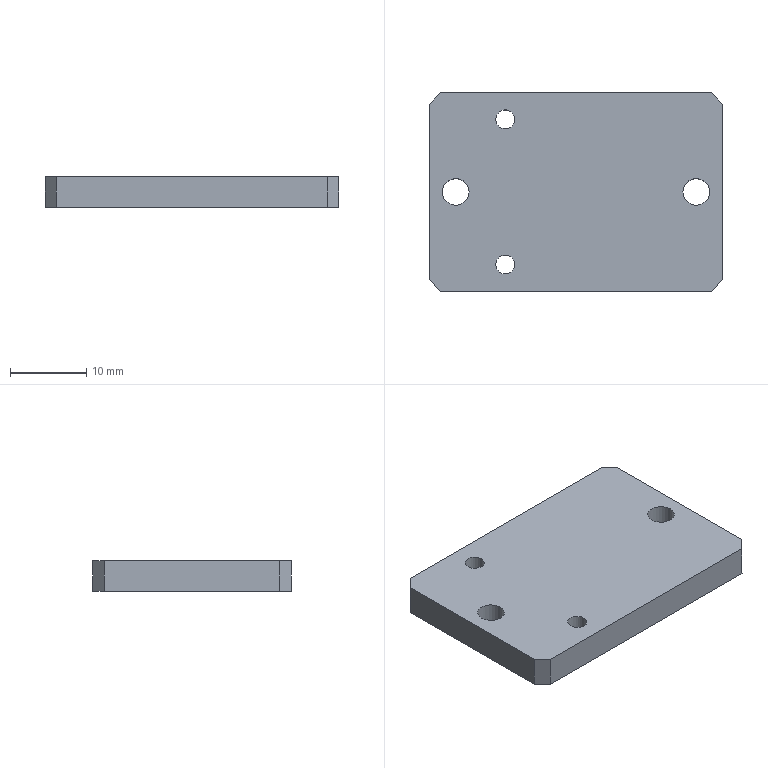Part | NX | 1 solid | 16 faces | box 38.5 x 26 x 4 mm | volume 3848 mm3 | plane 10 | cylinder 4 | cone 2 | commonest cylinder face diameters 2.5 x2 3.5 x2
STEP:
#1=CARTESIAN_POINT('',(19.25,-11.5,0.));
#2=VERTEX_POINT('',#1);
#3=CARTESIAN_POINT('',(19.25,11.5,0.));
#4=VERTEX_POINT('',#3);
#5=CARTESIAN_POINT('',(19.25,-13.,0.));
#6=DIRECTION('',(0.,1.,0.));
#7=VECTOR('',#6,1000.);
#8=LINE('',#5,#7);
#9=EDGE_CURVE('',#2,#4,#8,.T.);
#10=ORIENTED_EDGE('',*,*,#9,.T.);
#11=CARTESIAN_POINT('',(19.25,11.5,4.));
#12=VERTEX_POINT('',#11);
#13=CARTESIAN_POINT('',(19.25,11.5,4.));
#14=DIRECTION('',(0.,0.,1.));
#15=VECTOR('',#14,1000.);
#16=LINE('',#13,#15);
#17=EDGE_CURVE('',#4,#12,#16,.T.);
#18=ORIENTED_EDGE('',*,*,#17,.T.);
#19=CARTESIAN_POINT('',(19.25,-11.5,4.));
#20=VERTEX_POINT('',#19);
#21=CARTESIAN_POINT('',(19.25,-13.,4.));
#22=DIRECTION('',(0.,1.,0.));
#23=VECTOR('',#22,1000.);
#24=LINE('',#21,#23);
#25=EDGE_CURVE('',#20,#12,#24,.T.);
#26=ORIENTED_EDGE('',*,*,#25,.F.);
#27=CARTESIAN_POINT('',(19.25,-11.5,4.));
#28=DIRECTION('',(0.,0.,-1.));
#29=VECTOR('',#28,1000.);
#30=LINE('',#27,#29);
#31=EDGE_CURVE('',#20,#2,#30,.T.);
#32=ORIENTED_EDGE('',*,*,#31,.T.);
#33=EDGE_LOOP('',(#10,#18,#26,#32));
#34=FACE_BOUND('',#33,.T.);
#35=CARTESIAN_POINT('',(19.25,-13.,4.));
#36=DIRECTION('',(-1.,0.,0.));
#37=DIRECTION('',(0.,0.,1.));
#38=AXIS2_PLACEMENT_3D('',#35,#36,#37);
#39=PLANE('',#38);
#40=ADVANCED_FACE('',(#34),#39,.F.);
#41=CARTESIAN_POINT('',(17.75,13.,4.));
#42=VERTEX_POINT('',#41);
#43=CARTESIAN_POINT('',(-17.75,13.,4.));
#44=VERTEX_POINT('',#43);
#45=CARTESIAN_POINT('',(-19.25,13.,4.));
#46=DIRECTION('',(-1.,0.,0.));
#47=VECTOR('',#46,1000.);
#48=LINE('',#45,#47);
#49=EDGE_CURVE('',#42,#44,#48,.T.);
#50=ORIENTED_EDGE('',*,*,#49,.F.);
#51=CARTESIAN_POINT('',(17.75,13.,0.));
#52=VERTEX_POINT('',#51);
#53=CARTESIAN_POINT('',(17.75,13.,4.));
#54=DIRECTION('',(0.,0.,-1.));
#55=VECTOR('',#54,1000.);
#56=LINE('',#53,#55);
#57=EDGE_CURVE('',#42,#52,#56,.T.);
#58=ORIENTED_EDGE('',*,*,#57,.T.);
#59=CARTESIAN_POINT('',(-17.75,13.,0.));
#60=VERTEX_POINT('',#59);
#61=CARTESIAN_POINT('',(-19.25,13.,0.));
#62=DIRECTION('',(-1.,0.,0.));
#63=VECTOR('',#62,1000.);
#64=LINE('',#61,#63);
#65=EDGE_CURVE('',#52,#60,#64,.T.);
#66=ORIENTED_EDGE('',*,*,#65,.T.);
#67=CARTESIAN_POINT('',(-17.75,13.,4.));
#68=DIRECTION('',(0.,0.,1.));
#69=VECTOR('',#68,1000.);
#70=LINE('',#67,#69);
#71=EDGE_CURVE('',#60,#44,#70,.T.);
#72=ORIENTED_EDGE('',*,*,#71,.T.);
#73=EDGE_LOOP('',(#50,#58,#66,#72));
#74=FACE_BOUND('',#73,.T.);
#75=CARTESIAN_POINT('',(-19.25,13.,4.));
#76=DIRECTION('',(0.,-1.,0.));
#77=DIRECTION('',(0.,0.,-1.));
#78=AXIS2_PLACEMENT_3D('',#75,#76,#77);
#79=PLANE('',#78);
#80=ADVANCED_FACE('',(#74),#79,.F.);
#81=CARTESIAN_POINT('',(-19.25,11.5,0.));
#82=VERTEX_POINT('',#81);
#83=CARTESIAN_POINT('',(-19.25,-11.5,0.));
#84=VERTEX_POINT('',#83);
#85=CARTESIAN_POINT('',(-19.25,-13.,0.));
#86=DIRECTION('',(0.,-1.,0.));
#87=VECTOR('',#86,1000.);
#88=LINE('',#85,#87);
#89=EDGE_CURVE('',#82,#84,#88,.T.);
#90=ORIENTED_EDGE('',*,*,#89,.T.);
#91=CARTESIAN_POINT('',(-19.25,-11.5,4.));
#92=VERTEX_POINT('',#91);
#93=CARTESIAN_POINT('',(-19.25,-11.5,4.));
#94=DIRECTION('',(0.,0.,1.));
#95=VECTOR('',#94,1000.);
#96=LINE('',#93,#95);
#97=EDGE_CURVE('',#84,#92,#96,.T.);
#98=ORIENTED_EDGE('',*,*,#97,.T.);
#99=CARTESIAN_POINT('',(-19.25,11.5,4.));
#100=VERTEX_POINT('',#99);
#101=CARTESIAN_POINT('',(-19.25,-13.,4.));
#102=DIRECTION('',(0.,-1.,0.));
#103=VECTOR('',#102,1000.);
#104=LINE('',#101,#103);
#105=EDGE_CURVE('',#100,#92,#104,.T.);
#106=ORIENTED_EDGE('',*,*,#105,.F.);
#107=CARTESIAN_POINT('',(-19.25,11.5,4.));
#108=DIRECTION('',(0.,0.,-1.));
#109=VECTOR('',#108,1000.);
#110=LINE('',#107,#109);
#111=EDGE_CURVE('',#100,#82,#110,.T.);
#112=ORIENTED_EDGE('',*,*,#111,.T.);
#113=EDGE_LOOP('',(#90,#98,#106,#112));
#114=FACE_BOUND('',#113,.T.);
#115=CARTESIAN_POINT('',(-19.25,-13.,4.));
#116=DIRECTION('',(1.,0.,0.));
#117=DIRECTION('',(0.,0.,-1.));
#118=AXIS2_PLACEMENT_3D('',#115,#116,#117);
#119=PLANE('',#118);
#120=ADVANCED_FACE('',(#114),#119,.F.);
#121=CARTESIAN_POINT('',(-17.75,-13.,0.));
#122=VERTEX_POINT('',#121);
#123=CARTESIAN_POINT('',(17.75,-13.,0.));
#124=VERTEX_POINT('',#123);
#125=CARTESIAN_POINT('',(-19.25,-13.,0.));
#126=DIRECTION('',(1.,0.,0.));
#127=VECTOR('',#126,1000.);
#128=LINE('',#125,#127);
#129=EDGE_CURVE('',#122,#124,#128,.T.);
#130=ORIENTED_EDGE('',*,*,#129,.T.);
#131=CARTESIAN_POINT('',(17.75,-13.,4.));
#132=VERTEX_POINT('',#131);
#133=CARTESIAN_POINT('',(17.75,-13.,4.));
#134=DIRECTION('',(0.,0.,1.));
#135=VECTOR('',#134,1000.);
#136=LINE('',#133,#135);
#137=EDGE_CURVE('',#124,#132,#136,.T.);
#138=ORIENTED_EDGE('',*,*,#137,.T.);
#139=CARTESIAN_POINT('',(-17.75,-13.,4.));
#140=VERTEX_POINT('',#139);
#141=CARTESIAN_POINT('',(-19.25,-13.,4.));
#142=DIRECTION('',(1.,0.,0.));
#143=VECTOR('',#142,1000.);
#144=LINE('',#141,#143);
#145=EDGE_CURVE('',#140,#132,#144,.T.);
#146=ORIENTED_EDGE('',*,*,#145,.F.);
#147=CARTESIAN_POINT('',(-17.75,-13.,4.));
#148=DIRECTION('',(0.,0.,-1.));
#149=VECTOR('',#148,1000.);
#150=LINE('',#147,#149);
#151=EDGE_CURVE('',#140,#122,#150,.T.);
#152=ORIENTED_EDGE('',*,*,#151,.T.);
#153=EDGE_LOOP('',(#130,#138,#146,#152));
#154=FACE_BOUND('',#153,.T.);
#155=CARTESIAN_POINT('',(-19.25,-13.,4.));
#156=DIRECTION('',(0.,1.,0.));
#157=DIRECTION('',(0.,0.,1.));
#158=AXIS2_PLACEMENT_3D('',#155,#156,#157);
#159=PLANE('',#158);
#160=ADVANCED_FACE('',(#154),#159,.F.);
#161=CARTESIAN_POINT('',(-10.5,9.5,4.));
#162=VERTEX_POINT('',#161);
#163=CARTESIAN_POINT('',(-9.25,9.5,4.));
#164=DIRECTION('',(0.,0.,-1.));
#165=DIRECTION('',(-1.,0.,0.));
#166=AXIS2_PLACEMENT_3D('',#163,#164,#165);
#167=CIRCLE('',#166,1.25);
#168=EDGE_CURVE('',#162,#162,#167,.T.);
#169=ORIENTED_EDGE('',*,*,#168,.T.);
#170=EDGE_LOOP('',(#169));
#171=FACE_BOUND('',#170,.T.);
#172=CARTESIAN_POINT('',(-10.5,-9.5,4.));
#173=VERTEX_POINT('',#172);
#174=CARTESIAN_POINT('',(-9.25,-9.5,4.));
#175=DIRECTION('',(0.,0.,-1.));
#176=DIRECTION('',(-1.,0.,0.));
#177=AXIS2_PLACEMENT_3D('',#174,#175,#176);
#178=CIRCLE('',#177,1.25);
#179=EDGE_CURVE('',#173,#173,#178,.T.);
#180=ORIENTED_EDGE('',*,*,#179,.T.);
#181=EDGE_LOOP('',(#180));
#182=FACE_BOUND('',#181,.T.);
#183=CARTESIAN_POINT('',(14.,0.,4.));
#184=VERTEX_POINT('',#183);
#185=CARTESIAN_POINT('',(15.75,0.,4.));
#186=DIRECTION('',(0.,0.,-1.));
#187=DIRECTION('',(-1.,0.,0.));
#188=AXIS2_PLACEMENT_3D('',#185,#186,#187);
#189=CIRCLE('',#188,1.75);
#190=EDGE_CURVE('',#184,#184,#189,.T.);
#191=ORIENTED_EDGE('',*,*,#190,.T.);
#192=EDGE_LOOP('',(#191));
#193=FACE_BOUND('',#192,.T.);
#194=CARTESIAN_POINT('',(-17.5,0.,4.));
#195=VERTEX_POINT('',#194);
#196=CARTESIAN_POINT('',(-15.75,0.,4.));
#197=DIRECTION('',(0.,0.,-1.));
#198=DIRECTION('',(-1.,0.,0.));
#199=AXIS2_PLACEMENT_3D('',#196,#197,#198);
#200=CIRCLE('',#199,1.75);
#201=EDGE_CURVE('',#195,#195,#200,.T.);
#202=ORIENTED_EDGE('',*,*,#201,.T.);
#203=EDGE_LOOP('',(#202));
#204=FACE_BOUND('',#203,.T.);
#205=ORIENTED_EDGE('',*,*,#25,.T.);
#206=CARTESIAN_POINT('',(17.75,13.,4.));
#207=DIRECTION('',(0.7071,-0.7071,0.));
#208=VECTOR('',#207,1000.);
#209=LINE('',#206,#208);
#210=EDGE_CURVE('',#12,#42,#209,.F.);
#211=ORIENTED_EDGE('',*,*,#210,.T.);
#212=ORIENTED_EDGE('',*,*,#49,.T.);
#213=CARTESIAN_POINT('',(-19.25,11.5,4.));
#214=DIRECTION('',(0.7071,0.7071,0.));
#215=VECTOR('',#214,1000.);
#216=LINE('',#213,#215);
#217=EDGE_CURVE('',#44,#100,#216,.F.);
#218=ORIENTED_EDGE('',*,*,#217,.T.);
#219=ORIENTED_EDGE('',*,*,#105,.T.);
#220=CARTESIAN_POINT('',(-17.75,-13.,4.));
#221=DIRECTION('',(-0.7071,0.7071,0.));
#222=VECTOR('',#221,1000.);
#223=LINE('',#220,#222);
#224=EDGE_CURVE('',#92,#140,#223,.F.);
#225=ORIENTED_EDGE('',*,*,#224,.T.);
#226=ORIENTED_EDGE('',*,*,#145,.T.);
#227=CARTESIAN_POINT('',(19.25,-11.5,4.));
#228=DIRECTION('',(-0.7071,-0.7071,0.));
#229=VECTOR('',#228,1000.);
#230=LINE('',#227,#229);
#231=EDGE_CURVE('',#132,#20,#230,.F.);
#232=ORIENTED_EDGE('',*,*,#231,.T.);
#233=EDGE_LOOP('',(#205,#211,#212,#218,#219,#225,#226,#232));
#234=FACE_BOUND('',#233,.T.);
#235=CARTESIAN_POINT('',(0.,0.,4.));
#236=DIRECTION('',(0.,0.,-1.));
#237=DIRECTION('',(-1.,0.,0.));
#238=AXIS2_PLACEMENT_3D('',#235,#236,#237);
#239=PLANE('',#238);
#240=ADVANCED_FACE('',(#171,#182,#193,#204,#234),#239,.F.);
#241=CARTESIAN_POINT('',(-10.5,9.5,0.));
#242=VERTEX_POINT('',#241);
#243=CARTESIAN_POINT('',(-9.25,9.5,0.));
#244=DIRECTION('',(0.,0.,-1.));
#245=DIRECTION('',(-1.,0.,0.));
#246=AXIS2_PLACEMENT_3D('',#243,#244,#245);
#247=CIRCLE('',#246,1.25);
#248=EDGE_CURVE('',#242,#242,#247,.T.);
#249=ORIENTED_EDGE('',*,*,#248,.F.);
#250=EDGE_LOOP('',(#249));
#251=FACE_BOUND('',#250,.T.);
#252=CARTESIAN_POINT('',(-10.5,-9.5,0.));
#253=VERTEX_POINT('',#252);
#254=CARTESIAN_POINT('',(-9.25,-9.5,0.));
#255=DIRECTION('',(0.,0.,-1.));
#256=DIRECTION('',(-1.,0.,0.));
#257=AXIS2_PLACEMENT_3D('',#254,#255,#256);
#258=CIRCLE('',#257,1.25);
#259=EDGE_CURVE('',#253,#253,#258,.T.);
#260=ORIENTED_EDGE('',*,*,#259,.F.);
#261=EDGE_LOOP('',(#260));
#262=FACE_BOUND('',#261,.T.);
#263=CARTESIAN_POINT('',(12.75,0.,0.));
#264=VERTEX_POINT('',#263);
#265=CARTESIAN_POINT('',(15.75,0.,0.));
#266=DIRECTION('',(0.,0.,-1.));
#267=DIRECTION('',(-1.,0.,0.));
#268=AXIS2_PLACEMENT_3D('',#265,#266,#267);
#269=CIRCLE('',#268,3.);
#270=EDGE_CURVE('',#264,#264,#269,.T.);
#271=ORIENTED_EDGE('',*,*,#270,.F.);
#272=EDGE_LOOP('',(#271));
#273=FACE_BOUND('',#272,.T.);
#274=CARTESIAN_POINT('',(-18.75,0.,0.));
#275=VERTEX_POINT('',#274);
#276=CARTESIAN_POINT('',(-15.75,0.,0.));
#277=DIRECTION('',(0.,0.,-1.));
#278=DIRECTION('',(-1.,0.,0.));
#279=AXIS2_PLACEMENT_3D('',#276,#277,#278);
#280=CIRCLE('',#279,3.);
#281=EDGE_CURVE('',#275,#275,#280,.T.);
#282=ORIENTED_EDGE('',*,*,#281,.F.);
#283=EDGE_LOOP('',(#282));
#284=FACE_BOUND('',#283,.T.);
#285=ORIENTED_EDGE('',*,*,#65,.F.);
#286=CARTESIAN_POINT('',(15.375,15.375,0.));
#287=DIRECTION('',(-0.7071,0.7071,0.));
#288=VECTOR('',#287,1000.);
#289=LINE('',#286,#288);
#290=EDGE_CURVE('',#52,#4,#289,.F.);
#291=ORIENTED_EDGE('',*,*,#290,.T.);
#292=ORIENTED_EDGE('',*,*,#9,.F.);
#293=CARTESIAN_POINT('',(15.375,-15.375,0.));
#294=DIRECTION('',(0.7071,0.7071,0.));
#295=VECTOR('',#294,1000.);
#296=LINE('',#293,#295);
#297=EDGE_CURVE('',#2,#124,#296,.F.);
#298=ORIENTED_EDGE('',*,*,#297,.T.);
#299=ORIENTED_EDGE('',*,*,#129,.F.);
#300=CARTESIAN_POINT('',(-15.375,-15.375,0.));
#301=DIRECTION('',(0.7071,-0.7071,0.));
#302=VECTOR('',#301,1000.);
#303=LINE('',#300,#302);
#304=EDGE_CURVE('',#122,#84,#303,.F.);
#305=ORIENTED_EDGE('',*,*,#304,.T.);
#306=ORIENTED_EDGE('',*,*,#89,.F.);
#307=CARTESIAN_POINT('',(-15.375,15.375,0.));
#308=DIRECTION('',(-0.7071,-0.7071,0.));
#309=VECTOR('',#308,1000.);
#310=LINE('',#307,#309);
#311=EDGE_CURVE('',#82,#60,#310,.F.);
#312=ORIENTED_EDGE('',*,*,#311,.T.);
#313=EDGE_LOOP('',(#285,#291,#292,#298,#299,#305,#306,#312));
#314=FACE_BOUND('',#313,.T.);
#315=CARTESIAN_POINT('',(0.,0.,0.));
#316=DIRECTION('',(0.,0.,-1.));
#317=DIRECTION('',(-1.,0.,0.));
#318=AXIS2_PLACEMENT_3D('',#315,#316,#317);
#319=PLANE('',#318);
#320=ADVANCED_FACE('',(#251,#262,#273,#284,#314),#319,.T.);
#321=ORIENTED_EDGE('',*,*,#210,.F.);
#322=ORIENTED_EDGE('',*,*,#17,.F.);
#323=ORIENTED_EDGE('',*,*,#290,.F.);
#324=ORIENTED_EDGE('',*,*,#57,.F.);
#325=EDGE_LOOP('',(#321,#322,#323,#324));
#326=FACE_BOUND('',#325,.T.);
#327=CARTESIAN_POINT('',(17.75,13.,4.));
#328=DIRECTION('',(-0.7071,-0.7071,0.));
#329=DIRECTION('',(0.,0.,-1.));
#330=AXIS2_PLACEMENT_3D('',#327,#328,#329);
#331=PLANE('',#330);
#332=ADVANCED_FACE('',(#326),#331,.F.);
#333=ORIENTED_EDGE('',*,*,#231,.F.);
#334=ORIENTED_EDGE('',*,*,#137,.F.);
#335=ORIENTED_EDGE('',*,*,#297,.F.);
#336=ORIENTED_EDGE('',*,*,#31,.F.);
#337=EDGE_LOOP('',(#333,#334,#335,#336));
#338=FACE_BOUND('',#337,.T.);
#339=CARTESIAN_POINT('',(19.25,-11.5,4.));
#340=DIRECTION('',(-0.7071,0.7071,0.));
#341=DIRECTION('',(0.,0.,-1.));
#342=AXIS2_PLACEMENT_3D('',#339,#340,#341);
#343=PLANE('',#342);
#344=ADVANCED_FACE('',(#338),#343,.F.);
#345=ORIENTED_EDGE('',*,*,#224,.F.);
#346=ORIENTED_EDGE('',*,*,#97,.F.);
#347=ORIENTED_EDGE('',*,*,#304,.F.);
#348=ORIENTED_EDGE('',*,*,#151,.F.);
#349=EDGE_LOOP('',(#345,#346,#347,#348));
#350=FACE_BOUND('',#349,.T.);
#351=CARTESIAN_POINT('',(-17.75,-13.,4.));
#352=DIRECTION('',(0.7071,0.7071,0.));
#353=DIRECTION('',(0.,0.,-1.));
#354=AXIS2_PLACEMENT_3D('',#351,#352,#353);
#355=PLANE('',#354);
#356=ADVANCED_FACE('',(#350),#355,.F.);
#357=ORIENTED_EDGE('',*,*,#217,.F.);
#358=ORIENTED_EDGE('',*,*,#71,.F.);
#359=ORIENTED_EDGE('',*,*,#311,.F.);
#360=ORIENTED_EDGE('',*,*,#111,.F.);
#361=EDGE_LOOP('',(#357,#358,#359,#360));
#362=FACE_BOUND('',#361,.T.);
#363=CARTESIAN_POINT('',(-19.25,11.5,4.));
#364=DIRECTION('',(0.7071,-0.7071,0.));
#365=DIRECTION('',(0.,0.,-1.));
#366=AXIS2_PLACEMENT_3D('',#363,#364,#365);
#367=PLANE('',#366);
#368=ADVANCED_FACE('',(#362),#367,.F.);
#369=ORIENTED_EDGE('',*,*,#201,.F.);
#370=EDGE_LOOP('',(#369));
#371=FACE_BOUND('',#370,.T.);
#372=CARTESIAN_POINT('',(-17.5,0.,1.25));
#373=VERTEX_POINT('',#372);
#374=CARTESIAN_POINT('',(-15.75,0.,1.25));
#375=DIRECTION('',(0.,0.,-1.));
#376=DIRECTION('',(-1.,0.,0.));
#377=AXIS2_PLACEMENT_3D('',#374,#375,#376);
#378=CIRCLE('',#377,1.75);
#379=EDGE_CURVE('',#373,#373,#378,.T.);
#380=ORIENTED_EDGE('',*,*,#379,.T.);
#381=EDGE_LOOP('',(#380));
#382=FACE_BOUND('',#381,.T.);
#383=CARTESIAN_POINT('',(-15.75,0.,0.));
#384=DIRECTION('',(0.,0.,-1.));
#385=DIRECTION('',(-1.,0.,0.));
#386=AXIS2_PLACEMENT_3D('',#383,#384,#385);
#387=CYLINDRICAL_SURFACE('',#386,1.75);
#388=ADVANCED_FACE('',(#371,#382),#387,.F.);
#389=ORIENTED_EDGE('',*,*,#379,.F.);
#390=EDGE_LOOP('',(#389));
#391=FACE_BOUND('',#390,.T.);
#392=ORIENTED_EDGE('',*,*,#281,.T.);
#393=EDGE_LOOP('',(#392));
#394=FACE_BOUND('',#393,.T.);
#395=CARTESIAN_POINT('',(-15.75,0.,0.));
#396=DIRECTION('',(0.,0.,-1.));
#397=DIRECTION('',(-1.,0.,0.));
#398=AXIS2_PLACEMENT_3D('',#395,#396,#397);
#399=CONICAL_SURFACE('',#398,3.,0.7854);
#400=ADVANCED_FACE('',(#391,#394),#399,.F.);
#401=ORIENTED_EDGE('',*,*,#190,.F.);
#402=EDGE_LOOP('',(#401));
#403=FACE_BOUND('',#402,.T.);
#404=CARTESIAN_POINT('',(14.,0.,1.25));
#405=VERTEX_POINT('',#404);
#406=CARTESIAN_POINT('',(15.75,0.,1.25));
#407=DIRECTION('',(0.,0.,-1.));
#408=DIRECTION('',(-1.,0.,0.));
#409=AXIS2_PLACEMENT_3D('',#406,#407,#408);
#410=CIRCLE('',#409,1.75);
#411=EDGE_CURVE('',#405,#405,#410,.T.);
#412=ORIENTED_EDGE('',*,*,#411,.T.);
#413=EDGE_LOOP('',(#412));
#414=FACE_BOUND('',#413,.T.);
#415=CARTESIAN_POINT('',(15.75,0.,0.));
#416=DIRECTION('',(0.,0.,-1.));
#417=DIRECTION('',(-1.,0.,0.));
#418=AXIS2_PLACEMENT_3D('',#415,#416,#417);
#419=CYLINDRICAL_SURFACE('',#418,1.75);
#420=ADVANCED_FACE('',(#403,#414),#419,.F.);
#421=ORIENTED_EDGE('',*,*,#411,.F.);
#422=EDGE_LOOP('',(#421));
#423=FACE_BOUND('',#422,.T.);
#424=ORIENTED_EDGE('',*,*,#270,.T.);
#425=EDGE_LOOP('',(#424));
#426=FACE_BOUND('',#425,.T.);
#427=CARTESIAN_POINT('',(15.75,0.,0.));
#428=DIRECTION('',(0.,0.,-1.));
#429=DIRECTION('',(-1.,0.,0.));
#430=AXIS2_PLACEMENT_3D('',#427,#428,#429);
#431=CONICAL_SURFACE('',#430,3.,0.7854);
#432=ADVANCED_FACE('',(#423,#426),#431,.F.);
#433=ORIENTED_EDGE('',*,*,#179,.F.);
#434=EDGE_LOOP('',(#433));
#435=FACE_BOUND('',#434,.T.);
#436=ORIENTED_EDGE('',*,*,#259,.T.);
#437=EDGE_LOOP('',(#436));
#438=FACE_BOUND('',#437,.T.);
#439=CARTESIAN_POINT('',(-9.25,-9.5,0.));
#440=DIRECTION('',(0.,0.,-1.));
#441=DIRECTION('',(-1.,0.,0.));
#442=AXIS2_PLACEMENT_3D('',#439,#440,#441);
#443=CYLINDRICAL_SURFACE('',#442,1.25);
#444=ADVANCED_FACE('',(#435,#438),#443,.F.);
#445=ORIENTED_EDGE('',*,*,#168,.F.);
#446=EDGE_LOOP('',(#445));
#447=FACE_BOUND('',#446,.T.);
#448=ORIENTED_EDGE('',*,*,#248,.T.);
#449=EDGE_LOOP('',(#448));
#450=FACE_BOUND('',#449,.T.);
#451=CARTESIAN_POINT('',(-9.25,9.5,0.));
#452=DIRECTION('',(0.,0.,-1.));
#453=DIRECTION('',(-1.,0.,0.));
#454=AXIS2_PLACEMENT_3D('',#451,#452,#453);
#455=CYLINDRICAL_SURFACE('',#454,1.25);
#456=ADVANCED_FACE('',(#447,#450),#455,.F.);
#457=CLOSED_SHELL('',(#40,#80,#120,#160,#240,#320,#332,#344,#356,#368,#388,#400,#420,#432,#444,#456));
#458=MANIFOLD_SOLID_BREP('',#457);
#459=(LENGTH_UNIT()NAMED_UNIT(*)SI_UNIT(.MILLI.,.METRE.));
#460=UNCERTAINTY_MEASURE_WITH_UNIT(LENGTH_MEASURE(0.00001),#459,'','');
#461=(NAMED_UNIT(*)PLANE_ANGLE_UNIT()SI_UNIT($,.RADIAN.));
#462=(NAMED_UNIT(*)SI_UNIT($,.STERADIAN.)SOLID_ANGLE_UNIT());
#463=(GEOMETRIC_REPRESENTATION_CONTEXT(3)GLOBAL_UNCERTAINTY_ASSIGNED_CONTEXT((#460))GLOBAL_UNIT_ASSIGNED_CONTEXT((#459,#461,#462))REPRESENTATION_CONTEXT('',''));
#464=ADVANCED_BREP_SHAPE_REPRESENTATION('',(#458),#463);